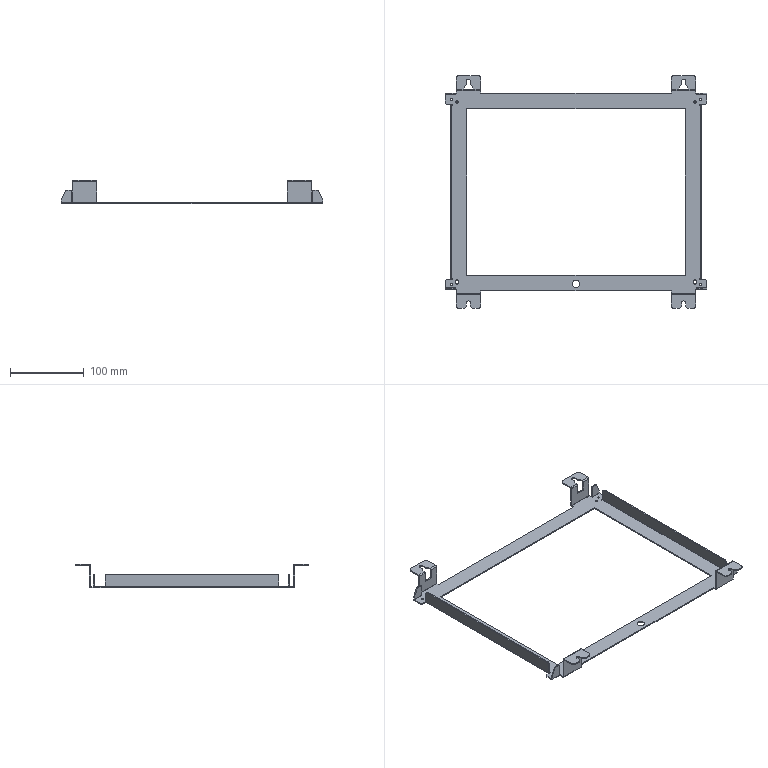Part | SolidWorks | features Jog 4, Chamfer 2, EdgeFlange 2, Fillet 1, FlatPattern 1, ICE 1, MirrorPattern 1, SMBaseFlange 1, SheetMetal 1 | 1 solid | 236 faces | box 354 x 314.5 x 31.5 mm | volume 59001 mm3 | plane 166 | cylinder 70 | commonest cylinder face diameters 0.4 x16 3.4 x16 6 x16 2.5 x8 3.2 x8 5.5 x4